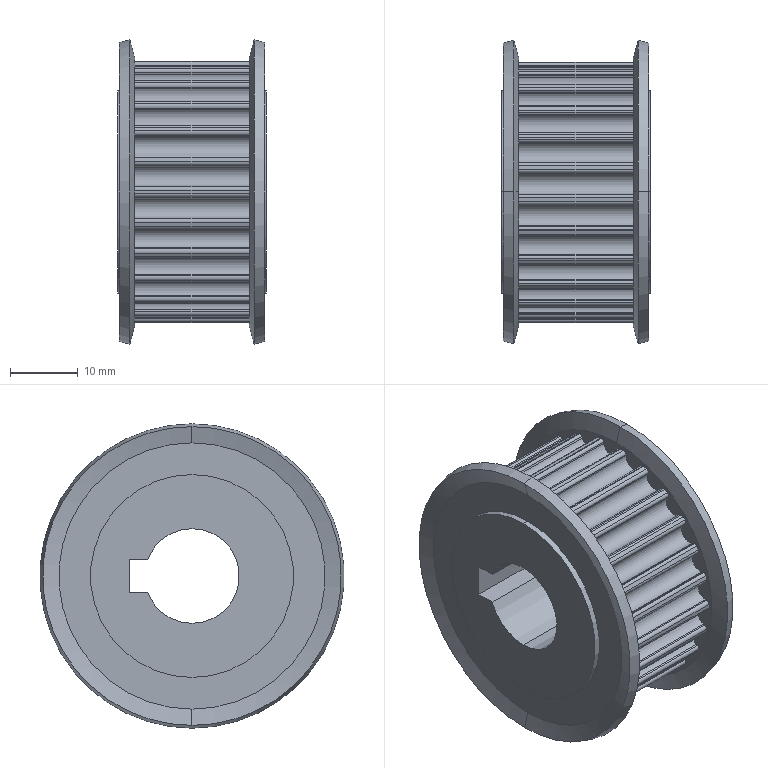Part | STEP file | C-HTPA25H5M150-A-N14 push-film drive pulley SGN-3-01 | 1 solid | 208 faces | box 22 x 45 x 45 mm | volume 20026 mm3 | cylinder 135 | plane 61 | cone 12 | commonest cylinder face diameters 1 x63 3.12 x38 38.65 x25 30 x4 14 x3 4.134 x2